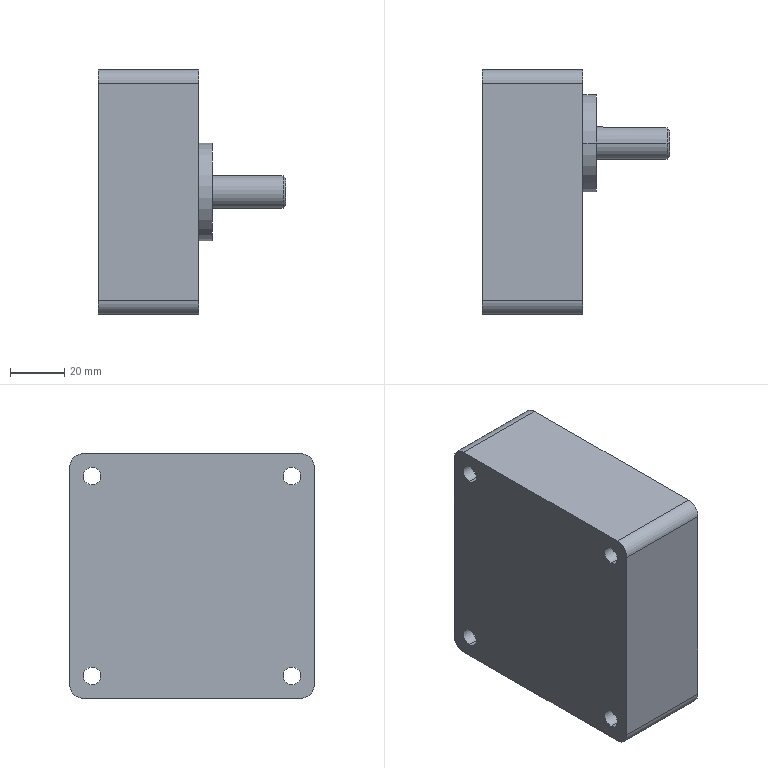Part | STEP file | 0230_Z_014_PACMGX90-3_1 | 1 solid | 31 faces | box 69 x 90 x 90 mm | volume 301887 mm3 | cylinder 17 | plane 11 | cone 3 | commonest cylinder face diameters 6.5 x8 10 x4 12 x2 36 x2 4 x1